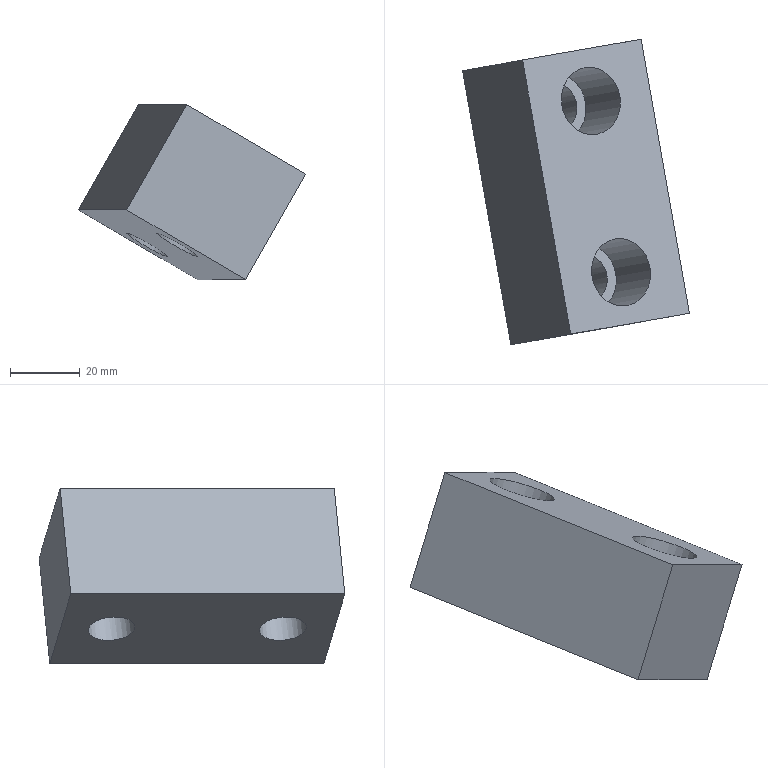Part | NX | features solid 2 | 1 solid | 12 faces | box 65.241 x 87.839 x 50.311 mm | volume 95760 mm3 | plane 8 | cylinder 4 | commonest cylinder face diameters 13.5 x2 19.5 x2
STEP:
#1=CARTESIAN_POINT('',(1073.315,75.129,-84.623));
#2=VERTEX_POINT('',#1);
#3=CARTESIAN_POINT('',(1087.206,-3.656,-84.623));
#4=VERTEX_POINT('',#3);
#5=CARTESIAN_POINT('',(1085.904,3.73,-84.623));
#6=DIRECTION('',(0.1736,-0.9848,0.));
#7=VECTOR('',#6,1000.);
#8=LINE('',#5,#7);
#9=EDGE_CURVE('',#2,#4,#8,.T.);
#10=ORIENTED_EDGE('',*,*,#9,.F.);
#11=CARTESIAN_POINT('',(1090.549,78.168,-54.312));
#12=VERTEX_POINT('',#11);
#13=CARTESIAN_POINT('',(1090.549,78.168,-54.312));
#14=DIRECTION('',(0.4924,0.08682,0.866));
#15=VECTOR('',#14,1000.);
#16=LINE('',#13,#15);
#17=EDGE_CURVE('',#2,#12,#16,.T.);
#18=ORIENTED_EDGE('',*,*,#17,.T.);
#19=CARTESIAN_POINT('',(1104.441,-0.617,-54.312));
#20=VERTEX_POINT('',#19);
#21=CARTESIAN_POINT('',(1103.138,6.769,-54.312));
#22=DIRECTION('',(0.1736,-0.9848,0.));
#23=VECTOR('',#22,1000.);
#24=LINE('',#21,#23);
#25=EDGE_CURVE('',#12,#20,#24,.T.);
#26=ORIENTED_EDGE('',*,*,#25,.T.);
#27=CARTESIAN_POINT('',(1104.441,-0.617,-54.312));
#28=DIRECTION('',(0.4924,0.08682,0.866));
#29=VECTOR('',#28,1000.);
#30=LINE('',#27,#29);
#31=EDGE_CURVE('',#4,#20,#30,.T.);
#32=ORIENTED_EDGE('',*,*,#31,.F.);
#33=EDGE_LOOP('',(#10,#18,#26,#32));
#34=FACE_BOUND('',#33,.T.);
#35=CARTESIAN_POINT('',(1103.138,6.769,-54.312));
#36=DIRECTION('',(0.8529,0.1504,-0.5));
#37=DIRECTION('',(-0.1736,0.9848,0.));
#38=AXIS2_PLACEMENT_3D('',#35,#36,#37);
#39=PLANE('',#38);
#40=ADVANCED_FACE('',(#34),#39,.T.);
#41=CARTESIAN_POINT('',(1056.434,72.152,-34.312));
#42=VERTEX_POINT('',#41);
#43=CARTESIAN_POINT('',(1060.272,72.829,-36.562));
#44=DIRECTION('',(0.8529,0.1504,-0.5));
#45=VECTOR('',#44,1000.);
#46=LINE('',#43,#45);
#47=EDGE_CURVE('',#42,#12,#46,.T.);
#48=ORIENTED_EDGE('',*,*,#47,.T.);
#49=ORIENTED_EDGE('',*,*,#17,.F.);
#50=CARTESIAN_POINT('',(1039.2,69.113,-64.623));
#51=VERTEX_POINT('',#50);
#52=CARTESIAN_POINT('',(1043.038,69.79,-66.873));
#53=DIRECTION('',(0.8529,0.1504,-0.5));
#54=VECTOR('',#53,1000.);
#55=LINE('',#52,#54);
#56=EDGE_CURVE('',#51,#2,#55,.T.);
#57=ORIENTED_EDGE('',*,*,#56,.F.);
#58=CARTESIAN_POINT('',(1056.434,72.152,-34.312));
#59=DIRECTION('',(-0.4924,-0.08682,-0.866));
#60=VECTOR('',#59,1000.);
#61=LINE('',#58,#60);
#62=EDGE_CURVE('',#42,#51,#61,.T.);
#63=ORIENTED_EDGE('',*,*,#62,.F.);
#64=EDGE_LOOP('',(#48,#49,#57,#63));
#65=FACE_BOUND('',#64,.T.);
#66=CARTESIAN_POINT('',(1060.272,72.829,-36.562));
#67=DIRECTION('',(0.1736,-0.9848,0.));
#68=DIRECTION('',(0.4924,0.08682,0.866));
#69=AXIS2_PLACEMENT_3D('',#66,#67,#68);
#70=PLANE('',#69);
#71=ADVANCED_FACE('',(#65),#70,.F.);
#72=CARTESIAN_POINT('',(1053.092,-9.671,-64.623));
#73=VERTEX_POINT('',#72);
#74=CARTESIAN_POINT('',(1051.789,-2.285,-64.623));
#75=DIRECTION('',(-0.1736,0.9848,0.));
#76=VECTOR('',#75,1000.);
#77=LINE('',#74,#76);
#78=EDGE_CURVE('',#73,#51,#77,.T.);
#79=ORIENTED_EDGE('',*,*,#78,.F.);
#80=CARTESIAN_POINT('',(1070.326,-6.632,-34.312));
#81=VERTEX_POINT('',#80);
#82=CARTESIAN_POINT('',(1070.326,-6.632,-34.312));
#83=DIRECTION('',(-0.4924,-0.08682,-0.866));
#84=VECTOR('',#83,1000.);
#85=LINE('',#82,#84);
#86=EDGE_CURVE('',#81,#73,#85,.T.);
#87=ORIENTED_EDGE('',*,*,#86,.F.);
#88=CARTESIAN_POINT('',(1069.024,0.7537,-34.312));
#89=DIRECTION('',(-0.1736,0.9848,0.));
#90=VECTOR('',#89,1000.);
#91=LINE('',#88,#90);
#92=EDGE_CURVE('',#81,#42,#91,.T.);
#93=ORIENTED_EDGE('',*,*,#92,.T.);
#94=ORIENTED_EDGE('',*,*,#62,.T.);
#95=EDGE_LOOP('',(#79,#87,#93,#94));
#96=FACE_BOUND('',#95,.T.);
#97=CARTESIAN_POINT('',(1069.024,0.7537,-34.312));
#98=DIRECTION('',(0.8529,0.1504,-0.5));
#99=DIRECTION('',(-0.1736,0.9848,0.));
#100=AXIS2_PLACEMENT_3D('',#97,#98,#99);
#101=PLANE('',#100);
#102=ADVANCED_FACE('',(#96),#101,.F.);
#103=CARTESIAN_POINT('',(1056.93,-8.994,-66.873));
#104=DIRECTION('',(0.8529,0.1504,-0.5));
#105=VECTOR('',#104,1000.);
#106=LINE('',#103,#105);
#107=EDGE_CURVE('',#73,#4,#106,.T.);
#108=ORIENTED_EDGE('',*,*,#107,.T.);
#109=ORIENTED_EDGE('',*,*,#31,.T.);
#110=CARTESIAN_POINT('',(1074.164,-5.956,-36.562));
#111=DIRECTION('',(0.8529,0.1504,-0.5));
#112=VECTOR('',#111,1000.);
#113=LINE('',#110,#112);
#114=EDGE_CURVE('',#81,#20,#113,.T.);
#115=ORIENTED_EDGE('',*,*,#114,.F.);
#116=ORIENTED_EDGE('',*,*,#86,.T.);
#117=EDGE_LOOP('',(#108,#109,#115,#116));
#118=FACE_BOUND('',#117,.T.);
#119=CARTESIAN_POINT('',(1074.164,-5.956,-36.562));
#120=DIRECTION('',(0.1736,-0.9848,0.));
#121=DIRECTION('',(0.4924,0.08682,0.866));
#122=AXIS2_PLACEMENT_3D('',#119,#120,#121);
#123=PLANE('',#122);
#124=ADVANCED_FACE('',(#118),#123,.T.);
#125=CARTESIAN_POINT('',(1092.743,14.046,-49.131));
#126=VERTEX_POINT('',#125);
#127=CARTESIAN_POINT('',(1084.779,11.147,-44.312));
#128=DIRECTION('',(0.4924,0.08682,0.866));
#129=DIRECTION('',(0.8169,0.2973,-0.4943));
#130=AXIS2_PLACEMENT_3D('',#127,#128,#129);
#131=CIRCLE('',#130,9.75);
#132=EDGE_CURVE('',#126,#126,#131,.T.);
#133=ORIENTED_EDGE('',*,*,#132,.F.);
#134=EDGE_LOOP('',(#133));
#135=FACE_BOUND('',#134,.T.);
#136=CARTESIAN_POINT('',(1084.061,63.287,-49.131));
#137=VERTEX_POINT('',#136);
#138=CARTESIAN_POINT('',(1076.096,60.388,-44.312));
#139=DIRECTION('',(0.4924,0.08682,0.866));
#140=DIRECTION('',(0.8169,0.2973,-0.4943));
#141=AXIS2_PLACEMENT_3D('',#138,#139,#140);
#142=CIRCLE('',#141,9.75);
#143=EDGE_CURVE('',#137,#137,#142,.T.);
#144=ORIENTED_EDGE('',*,*,#143,.F.);
#145=EDGE_LOOP('',(#144));
#146=FACE_BOUND('',#145,.T.);
#147=ORIENTED_EDGE('',*,*,#47,.F.);
#148=ORIENTED_EDGE('',*,*,#92,.F.);
#149=ORIENTED_EDGE('',*,*,#114,.T.);
#150=ORIENTED_EDGE('',*,*,#25,.F.);
#151=EDGE_LOOP('',(#147,#148,#149,#150));
#152=FACE_BOUND('',#151,.T.);
#153=CARTESIAN_POINT('',(1072.861,1.43,-36.562));
#154=DIRECTION('',(0.4924,0.08682,0.866));
#155=DIRECTION('',(-0.8529,-0.1504,0.5));
#156=AXIS2_PLACEMENT_3D('',#153,#154,#155);
#157=PLANE('',#156);
#158=ADVANCED_FACE('',(#135,#146,#152),#157,.T.);
#159=CARTESIAN_POINT('',(1073.417,7.971,-77.948));
#160=VERTEX_POINT('',#159);
#161=CARTESIAN_POINT('',(1067.544,8.109,-74.623));
#162=DIRECTION('',(0.4924,0.08682,0.866));
#163=DIRECTION('',(0.87,-0.02032,-0.4926));
#164=AXIS2_PLACEMENT_3D('',#161,#162,#163);
#165=CIRCLE('',#164,6.75);
#166=EDGE_CURVE('',#160,#160,#165,.F.);
#167=ORIENTED_EDGE('',*,*,#166,.F.);
#168=EDGE_LOOP('',(#167));
#169=FACE_BOUND('',#168,.T.);
#170=CARTESIAN_POINT('',(1064.734,57.212,-77.948));
#171=VERTEX_POINT('',#170);
#172=CARTESIAN_POINT('',(1058.862,57.349,-74.623));
#173=DIRECTION('',(0.4924,0.08682,0.866));
#174=DIRECTION('',(0.87,-0.02032,-0.4926));
#175=AXIS2_PLACEMENT_3D('',#172,#173,#174);
#176=CIRCLE('',#175,6.75);
#177=EDGE_CURVE('',#171,#171,#176,.F.);
#178=ORIENTED_EDGE('',*,*,#177,.F.);
#179=EDGE_LOOP('',(#178));
#180=FACE_BOUND('',#179,.T.);
#181=ORIENTED_EDGE('',*,*,#56,.T.);
#182=ORIENTED_EDGE('',*,*,#9,.T.);
#183=ORIENTED_EDGE('',*,*,#107,.F.);
#184=ORIENTED_EDGE('',*,*,#78,.T.);
#185=EDGE_LOOP('',(#181,#182,#183,#184));
#186=FACE_BOUND('',#185,.T.);
#187=CARTESIAN_POINT('',(1055.627,-1.608,-66.873));
#188=DIRECTION('',(0.4924,0.08682,0.866));
#189=DIRECTION('',(-0.8529,-0.1504,0.5));
#190=AXIS2_PLACEMENT_3D('',#187,#188,#189);
#191=PLANE('',#190);
#192=ADVANCED_FACE('',(#169,#180,#186),#191,.F.);
#193=CARTESIAN_POINT('',(1060.734,56.644,-58.296));
#194=VERTEX_POINT('',#193);
#195=CARTESIAN_POINT('',(1066.248,58.651,-61.632));
#196=DIRECTION('',(-0.4924,-0.08682,-0.866));
#197=DIRECTION('',(-0.8169,-0.2973,0.4943));
#198=AXIS2_PLACEMENT_3D('',#195,#196,#197);
#199=CIRCLE('',#198,6.75);
#200=EDGE_CURVE('',#194,#194,#199,.F.);
#201=ORIENTED_EDGE('',*,*,#200,.T.);
#202=EDGE_LOOP('',(#201));
#203=FACE_BOUND('',#202,.T.);
#204=ORIENTED_EDGE('',*,*,#177,.T.);
#205=EDGE_LOOP('',(#204));
#206=FACE_BOUND('',#205,.T.);
#207=CARTESIAN_POINT('',(1051.476,56.047,-87.613));
#208=DIRECTION('',(-0.4924,-0.08682,-0.866));
#209=DIRECTION('',(-0.8106,-0.3167,0.4926));
#210=AXIS2_PLACEMENT_3D('',#207,#208,#209);
#211=CYLINDRICAL_SURFACE('',#210,6.75);
#212=ADVANCED_FACE('',(#203,#206),#211,.F.);
#213=ORIENTED_EDGE('',*,*,#200,.F.);
#214=EDGE_LOOP('',(#213));
#215=FACE_BOUND('',#214,.T.);
#216=CARTESIAN_POINT('',(1058.283,55.752,-56.813));
#217=VERTEX_POINT('',#216);
#218=CARTESIAN_POINT('',(1066.248,58.651,-61.632));
#219=DIRECTION('',(-0.4924,-0.08682,-0.866));
#220=DIRECTION('',(-0.8169,-0.2973,0.4943));
#221=AXIS2_PLACEMENT_3D('',#218,#219,#220);
#222=CIRCLE('',#221,9.75);
#223=EDGE_CURVE('',#217,#217,#222,.F.);
#224=ORIENTED_EDGE('',*,*,#223,.T.);
#225=EDGE_LOOP('',(#224));
#226=FACE_BOUND('',#225,.T.);
#227=CARTESIAN_POINT('',(1067.985,48.803,-61.632));
#228=DIRECTION('',(-0.4924,-0.08682,-0.866));
#229=DIRECTION('',(-0.8106,-0.3167,0.4926));
#230=AXIS2_PLACEMENT_3D('',#227,#228,#229);
#231=PLANE('',#230);
#232=ADVANCED_FACE('',(#215,#226),#231,.F.);
#233=ORIENTED_EDGE('',*,*,#223,.F.);
#234=EDGE_LOOP('',(#233));
#235=FACE_BOUND('',#234,.T.);
#236=ORIENTED_EDGE('',*,*,#143,.T.);
#237=EDGE_LOOP('',(#236));
#238=FACE_BOUND('',#237,.T.);
#239=CARTESIAN_POINT('',(1076.096,60.388,-44.312));
#240=DIRECTION('',(-0.4924,-0.08682,-0.866));
#241=DIRECTION('',(-0.8106,-0.3167,0.4926));
#242=AXIS2_PLACEMENT_3D('',#239,#240,#241);
#243=CYLINDRICAL_SURFACE('',#242,9.75);
#244=ADVANCED_FACE('',(#235,#238),#243,.F.);
#245=CARTESIAN_POINT('',(1069.416,7.404,-58.296));
#246=VERTEX_POINT('',#245);
#247=CARTESIAN_POINT('',(1074.93,9.411,-61.632));
#248=DIRECTION('',(-0.4924,-0.08682,-0.866));
#249=DIRECTION('',(-0.8169,-0.2973,0.4943));
#250=AXIS2_PLACEMENT_3D('',#247,#248,#249);
#251=CIRCLE('',#250,6.75);
#252=EDGE_CURVE('',#246,#246,#251,.F.);
#253=ORIENTED_EDGE('',*,*,#252,.T.);
#254=EDGE_LOOP('',(#253));
#255=FACE_BOUND('',#254,.T.);
#256=ORIENTED_EDGE('',*,*,#166,.T.);
#257=EDGE_LOOP('',(#256));
#258=FACE_BOUND('',#257,.T.);
#259=CARTESIAN_POINT('',(1060.158,6.806,-87.613));
#260=DIRECTION('',(-0.4924,-0.08682,-0.866));
#261=DIRECTION('',(-0.8106,-0.3167,0.4926));
#262=AXIS2_PLACEMENT_3D('',#259,#260,#261);
#263=CYLINDRICAL_SURFACE('',#262,6.75);
#264=ADVANCED_FACE('',(#255,#258),#263,.F.);
#265=ORIENTED_EDGE('',*,*,#252,.F.);
#266=EDGE_LOOP('',(#265));
#267=FACE_BOUND('',#266,.T.);
#268=CARTESIAN_POINT('',(1066.966,6.512,-56.813));
#269=VERTEX_POINT('',#268);
#270=CARTESIAN_POINT('',(1074.93,9.411,-61.632));
#271=DIRECTION('',(-0.4924,-0.08682,-0.866));
#272=DIRECTION('',(-0.8169,-0.2973,0.4943));
#273=AXIS2_PLACEMENT_3D('',#270,#271,#272);
#274=CIRCLE('',#273,9.75);
#275=EDGE_CURVE('',#269,#269,#274,.F.);
#276=ORIENTED_EDGE('',*,*,#275,.T.);
#277=EDGE_LOOP('',(#276));
#278=FACE_BOUND('',#277,.T.);
#279=CARTESIAN_POINT('',(1073.194,19.259,-61.632));
#280=DIRECTION('',(-0.4924,-0.08682,-0.866));
#281=DIRECTION('',(-0.8106,-0.3167,0.4926));
#282=AXIS2_PLACEMENT_3D('',#279,#280,#281);
#283=PLANE('',#282);
#284=ADVANCED_FACE('',(#267,#278),#283,.F.);
#285=ORIENTED_EDGE('',*,*,#275,.F.);
#286=EDGE_LOOP('',(#285));
#287=FACE_BOUND('',#286,.T.);
#288=ORIENTED_EDGE('',*,*,#132,.T.);
#289=EDGE_LOOP('',(#288));
#290=FACE_BOUND('',#289,.T.);
#291=CARTESIAN_POINT('',(1084.779,11.147,-44.312));
#292=DIRECTION('',(-0.4924,-0.08682,-0.866));
#293=DIRECTION('',(-0.8106,-0.3167,0.4926));
#294=AXIS2_PLACEMENT_3D('',#291,#292,#293);
#295=CYLINDRICAL_SURFACE('',#294,9.75);
#296=ADVANCED_FACE('',(#287,#290),#295,.F.);
#297=CLOSED_SHELL('',(#40,#71,#102,#124,#158,#192,#212,#232,#244,#264,#284,#296));
#298=MANIFOLD_SOLID_BREP('',#297);
#299=(LENGTH_UNIT()NAMED_UNIT(*)SI_UNIT(.MILLI.,.METRE.));
#300=UNCERTAINTY_MEASURE_WITH_UNIT(LENGTH_MEASURE(0.00001),#299,'','');
#301=(NAMED_UNIT(*)PLANE_ANGLE_UNIT()SI_UNIT($,.RADIAN.));
#302=(NAMED_UNIT(*)SI_UNIT($,.STERADIAN.)SOLID_ANGLE_UNIT());
#303=(GEOMETRIC_REPRESENTATION_CONTEXT(3)GLOBAL_UNCERTAINTY_ASSIGNED_CONTEXT((#300))GLOBAL_UNIT_ASSIGNED_CONTEXT((#299,#301,#302))REPRESENTATION_CONTEXT('',''));
#304=ADVANCED_BREP_SHAPE_REPRESENTATION('',(#298),#303);